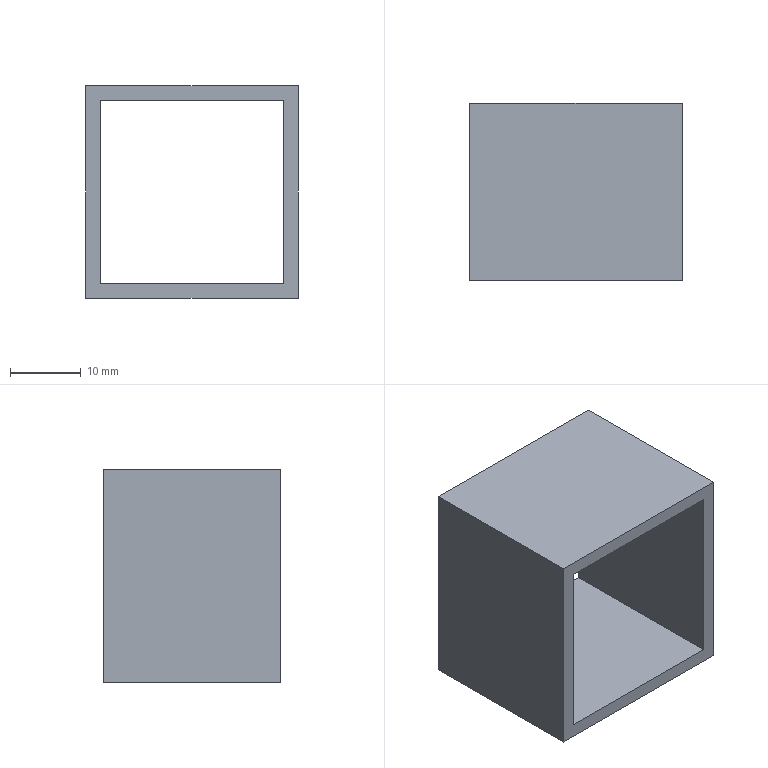Part | NX | features solid 2 | 1 solid | 10 faces | box 30 x 25 x 30 mm | volume 5600 mm3 | plane 10
STEP:
#1=CARTESIAN_POINT('',(350.,325.,-45.));
#2=VERTEX_POINT('',#1);
#3=CARTESIAN_POINT('',(380.,325.,-45.));
#4=VERTEX_POINT('',#3);
#5=CARTESIAN_POINT('',(350.,325.,-45.));
#6=DIRECTION('',(-1.,0.,0.));
#7=VECTOR('',#6,1000.);
#8=LINE('',#5,#7);
#9=EDGE_CURVE('',#2,#4,#8,.F.);
#10=ORIENTED_EDGE('',*,*,#9,.F.);
#11=CARTESIAN_POINT('',(350.,300.,-45.));
#12=VERTEX_POINT('',#11);
#13=CARTESIAN_POINT('',(350.,325.,-45.));
#14=DIRECTION('',(0.,-1.,0.));
#15=VECTOR('',#14,1000.);
#16=LINE('',#13,#15);
#17=EDGE_CURVE('',#2,#12,#16,.T.);
#18=ORIENTED_EDGE('',*,*,#17,.T.);
#19=CARTESIAN_POINT('',(380.,300.,-45.));
#20=VERTEX_POINT('',#19);
#21=CARTESIAN_POINT('',(350.,300.,-45.));
#22=DIRECTION('',(-1.,0.,0.));
#23=VECTOR('',#22,1000.);
#24=LINE('',#21,#23);
#25=EDGE_CURVE('',#12,#20,#24,.F.);
#26=ORIENTED_EDGE('',*,*,#25,.T.);
#27=CARTESIAN_POINT('',(380.,325.,-45.));
#28=DIRECTION('',(0.,-1.,0.));
#29=VECTOR('',#28,1000.);
#30=LINE('',#27,#29);
#31=EDGE_CURVE('',#4,#20,#30,.T.);
#32=ORIENTED_EDGE('',*,*,#31,.F.);
#33=EDGE_LOOP('',(#10,#18,#26,#32));
#34=FACE_BOUND('',#33,.T.);
#35=CARTESIAN_POINT('',(350.,325.,-45.));
#36=DIRECTION('',(0.,0.,-1.));
#37=DIRECTION('',(1.,0.,0.));
#38=AXIS2_PLACEMENT_3D('',#35,#36,#37);
#39=PLANE('',#38);
#40=ADVANCED_FACE('',(#34),#39,.F.);
#41=CARTESIAN_POINT('',(380.,325.,-75.));
#42=VERTEX_POINT('',#41);
#43=CARTESIAN_POINT('',(380.,325.,-45.));
#44=DIRECTION('',(0.,0.,1.));
#45=VECTOR('',#44,1000.);
#46=LINE('',#43,#45);
#47=EDGE_CURVE('',#4,#42,#46,.F.);
#48=ORIENTED_EDGE('',*,*,#47,.F.);
#49=ORIENTED_EDGE('',*,*,#31,.T.);
#50=CARTESIAN_POINT('',(380.,300.,-75.));
#51=VERTEX_POINT('',#50);
#52=CARTESIAN_POINT('',(380.,300.,-45.));
#53=DIRECTION('',(0.,0.,1.));
#54=VECTOR('',#53,1000.);
#55=LINE('',#52,#54);
#56=EDGE_CURVE('',#20,#51,#55,.F.);
#57=ORIENTED_EDGE('',*,*,#56,.T.);
#58=CARTESIAN_POINT('',(380.,325.,-75.));
#59=DIRECTION('',(0.,-1.,0.));
#60=VECTOR('',#59,1000.);
#61=LINE('',#58,#60);
#62=EDGE_CURVE('',#42,#51,#61,.T.);
#63=ORIENTED_EDGE('',*,*,#62,.F.);
#64=EDGE_LOOP('',(#48,#49,#57,#63));
#65=FACE_BOUND('',#64,.T.);
#66=CARTESIAN_POINT('',(380.,325.,-45.));
#67=DIRECTION('',(-1.,0.,0.));
#68=DIRECTION('',(0.,0.,-1.));
#69=AXIS2_PLACEMENT_3D('',#66,#67,#68);
#70=PLANE('',#69);
#71=ADVANCED_FACE('',(#65),#70,.F.);
#72=CARTESIAN_POINT('',(350.,325.,-75.));
#73=VERTEX_POINT('',#72);
#74=CARTESIAN_POINT('',(350.,325.,-75.));
#75=DIRECTION('',(-1.,0.,0.));
#76=VECTOR('',#75,1000.);
#77=LINE('',#74,#76);
#78=EDGE_CURVE('',#42,#73,#77,.T.);
#79=ORIENTED_EDGE('',*,*,#78,.F.);
#80=ORIENTED_EDGE('',*,*,#62,.T.);
#81=CARTESIAN_POINT('',(350.,300.,-75.));
#82=VERTEX_POINT('',#81);
#83=CARTESIAN_POINT('',(25.,300.,-75.));
#84=DIRECTION('',(1.,0.,0.));
#85=VECTOR('',#84,1000.);
#86=LINE('',#83,#85);
#87=EDGE_CURVE('',#82,#51,#86,.T.);
#88=ORIENTED_EDGE('',*,*,#87,.F.);
#89=CARTESIAN_POINT('',(350.,325.,-75.));
#90=DIRECTION('',(0.,-1.,0.));
#91=VECTOR('',#90,1000.);
#92=LINE('',#89,#91);
#93=EDGE_CURVE('',#73,#82,#92,.T.);
#94=ORIENTED_EDGE('',*,*,#93,.F.);
#95=EDGE_LOOP('',(#79,#80,#88,#94));
#96=FACE_BOUND('',#95,.T.);
#97=CARTESIAN_POINT('',(350.,325.,-75.));
#98=DIRECTION('',(0.,0.,-1.));
#99=DIRECTION('',(1.,0.,0.));
#100=AXIS2_PLACEMENT_3D('',#97,#98,#99);
#101=PLANE('',#100);
#102=ADVANCED_FACE('',(#96),#101,.T.);
#103=CARTESIAN_POINT('',(350.,325.,-45.));
#104=DIRECTION('',(0.,0.,1.));
#105=VECTOR('',#104,1000.);
#106=LINE('',#103,#105);
#107=EDGE_CURVE('',#73,#2,#106,.T.);
#108=ORIENTED_EDGE('',*,*,#107,.F.);
#109=ORIENTED_EDGE('',*,*,#93,.T.);
#110=CARTESIAN_POINT('',(350.,300.,-45.));
#111=DIRECTION('',(0.,0.,-1.));
#112=VECTOR('',#111,1000.);
#113=LINE('',#110,#112);
#114=EDGE_CURVE('',#12,#82,#113,.T.);
#115=ORIENTED_EDGE('',*,*,#114,.F.);
#116=ORIENTED_EDGE('',*,*,#17,.F.);
#117=EDGE_LOOP('',(#108,#109,#115,#116));
#118=FACE_BOUND('',#117,.T.);
#119=CARTESIAN_POINT('',(350.,325.,-45.));
#120=DIRECTION('',(-1.,0.,0.));
#121=DIRECTION('',(0.,0.,-1.));
#122=AXIS2_PLACEMENT_3D('',#119,#120,#121);
#123=PLANE('',#122);
#124=ADVANCED_FACE('',(#118),#123,.T.);
#125=ORIENTED_EDGE('',*,*,#56,.F.);
#126=ORIENTED_EDGE('',*,*,#25,.F.);
#127=ORIENTED_EDGE('',*,*,#114,.T.);
#128=ORIENTED_EDGE('',*,*,#87,.T.);
#129=EDGE_LOOP('',(#125,#126,#127,#128));
#130=FACE_BOUND('',#129,.T.);
#131=CARTESIAN_POINT('',(352.,300.,-47.));
#132=VERTEX_POINT('',#131);
#133=CARTESIAN_POINT('',(378.,300.,-47.));
#134=VERTEX_POINT('',#133);
#135=CARTESIAN_POINT('',(350.,300.,-47.));
#136=DIRECTION('',(-1.,0.,0.));
#137=VECTOR('',#136,1000.);
#138=LINE('',#135,#137);
#139=EDGE_CURVE('',#132,#134,#138,.F.);
#140=ORIENTED_EDGE('',*,*,#139,.T.);
#141=CARTESIAN_POINT('',(378.,300.,-73.));
#142=VERTEX_POINT('',#141);
#143=CARTESIAN_POINT('',(378.,300.,-45.));
#144=DIRECTION('',(0.,0.,1.));
#145=VECTOR('',#144,1000.);
#146=LINE('',#143,#145);
#147=EDGE_CURVE('',#134,#142,#146,.F.);
#148=ORIENTED_EDGE('',*,*,#147,.T.);
#149=CARTESIAN_POINT('',(352.,300.,-73.));
#150=VERTEX_POINT('',#149);
#151=CARTESIAN_POINT('',(25.,300.,-73.));
#152=DIRECTION('',(1.,0.,0.));
#153=VECTOR('',#152,1000.);
#154=LINE('',#151,#153);
#155=EDGE_CURVE('',#150,#142,#154,.T.);
#156=ORIENTED_EDGE('',*,*,#155,.F.);
#157=CARTESIAN_POINT('',(352.,300.,-45.));
#158=DIRECTION('',(0.,0.,-1.));
#159=VECTOR('',#158,1000.);
#160=LINE('',#157,#159);
#161=EDGE_CURVE('',#132,#150,#160,.T.);
#162=ORIENTED_EDGE('',*,*,#161,.F.);
#163=EDGE_LOOP('',(#140,#148,#156,#162));
#164=FACE_BOUND('',#163,.T.);
#165=CARTESIAN_POINT('',(25.,300.,-45.));
#166=DIRECTION('',(0.,-1.,0.));
#167=DIRECTION('',(1.,0.,0.));
#168=AXIS2_PLACEMENT_3D('',#165,#166,#167);
#169=PLANE('',#168);
#170=ADVANCED_FACE('',(#130,#164),#169,.T.);
#171=CARTESIAN_POINT('',(352.,325.,-47.));
#172=VERTEX_POINT('',#171);
#173=CARTESIAN_POINT('',(352.,325.,-47.));
#174=DIRECTION('',(0.,1.,0.));
#175=VECTOR('',#174,1000.);
#176=LINE('',#173,#175);
#177=EDGE_CURVE('',#172,#132,#176,.F.);
#178=ORIENTED_EDGE('',*,*,#177,.F.);
#179=CARTESIAN_POINT('',(378.,325.,-47.));
#180=VERTEX_POINT('',#179);
#181=CARTESIAN_POINT('',(350.,325.,-47.));
#182=DIRECTION('',(-1.,0.,0.));
#183=VECTOR('',#182,1000.);
#184=LINE('',#181,#183);
#185=EDGE_CURVE('',#172,#180,#184,.F.);
#186=ORIENTED_EDGE('',*,*,#185,.T.);
#187=CARTESIAN_POINT('',(378.,325.,-47.));
#188=DIRECTION('',(0.,-1.,0.));
#189=VECTOR('',#188,1000.);
#190=LINE('',#187,#189);
#191=EDGE_CURVE('',#180,#134,#190,.T.);
#192=ORIENTED_EDGE('',*,*,#191,.T.);
#193=ORIENTED_EDGE('',*,*,#139,.F.);
#194=EDGE_LOOP('',(#178,#186,#192,#193));
#195=FACE_BOUND('',#194,.T.);
#196=CARTESIAN_POINT('',(350.,325.,-47.));
#197=DIRECTION('',(0.,0.,-1.));
#198=DIRECTION('',(1.,0.,0.));
#199=AXIS2_PLACEMENT_3D('',#196,#197,#198);
#200=PLANE('',#199);
#201=ADVANCED_FACE('',(#195),#200,.T.);
#202=ORIENTED_EDGE('',*,*,#191,.F.);
#203=CARTESIAN_POINT('',(378.,325.,-73.));
#204=VERTEX_POINT('',#203);
#205=CARTESIAN_POINT('',(378.,325.,-45.));
#206=DIRECTION('',(0.,0.,1.));
#207=VECTOR('',#206,1000.);
#208=LINE('',#205,#207);
#209=EDGE_CURVE('',#180,#204,#208,.F.);
#210=ORIENTED_EDGE('',*,*,#209,.T.);
#211=CARTESIAN_POINT('',(378.,325.,-73.));
#212=DIRECTION('',(0.,1.,0.));
#213=VECTOR('',#212,1000.);
#214=LINE('',#211,#213);
#215=EDGE_CURVE('',#204,#142,#214,.F.);
#216=ORIENTED_EDGE('',*,*,#215,.T.);
#217=ORIENTED_EDGE('',*,*,#147,.F.);
#218=EDGE_LOOP('',(#202,#210,#216,#217));
#219=FACE_BOUND('',#218,.T.);
#220=CARTESIAN_POINT('',(378.,325.,-45.));
#221=DIRECTION('',(-1.,0.,0.));
#222=DIRECTION('',(0.,0.,-1.));
#223=AXIS2_PLACEMENT_3D('',#220,#221,#222);
#224=PLANE('',#223);
#225=ADVANCED_FACE('',(#219),#224,.T.);
#226=ORIENTED_EDGE('',*,*,#215,.F.);
#227=CARTESIAN_POINT('',(352.,325.,-73.));
#228=VERTEX_POINT('',#227);
#229=CARTESIAN_POINT('',(350.,325.,-73.));
#230=DIRECTION('',(-1.,0.,0.));
#231=VECTOR('',#230,1000.);
#232=LINE('',#229,#231);
#233=EDGE_CURVE('',#204,#228,#232,.T.);
#234=ORIENTED_EDGE('',*,*,#233,.T.);
#235=CARTESIAN_POINT('',(352.,325.,-73.));
#236=DIRECTION('',(0.,-1.,0.));
#237=VECTOR('',#236,1000.);
#238=LINE('',#235,#237);
#239=EDGE_CURVE('',#228,#150,#238,.T.);
#240=ORIENTED_EDGE('',*,*,#239,.T.);
#241=ORIENTED_EDGE('',*,*,#155,.T.);
#242=EDGE_LOOP('',(#226,#234,#240,#241));
#243=FACE_BOUND('',#242,.T.);
#244=CARTESIAN_POINT('',(350.,325.,-73.));
#245=DIRECTION('',(0.,0.,-1.));
#246=DIRECTION('',(1.,0.,0.));
#247=AXIS2_PLACEMENT_3D('',#244,#245,#246);
#248=PLANE('',#247);
#249=ADVANCED_FACE('',(#243),#248,.F.);
#250=ORIENTED_EDGE('',*,*,#239,.F.);
#251=CARTESIAN_POINT('',(352.,325.,-45.));
#252=DIRECTION('',(0.,0.,1.));
#253=VECTOR('',#252,1000.);
#254=LINE('',#251,#253);
#255=EDGE_CURVE('',#228,#172,#254,.T.);
#256=ORIENTED_EDGE('',*,*,#255,.T.);
#257=ORIENTED_EDGE('',*,*,#177,.T.);
#258=ORIENTED_EDGE('',*,*,#161,.T.);
#259=EDGE_LOOP('',(#250,#256,#257,#258));
#260=FACE_BOUND('',#259,.T.);
#261=CARTESIAN_POINT('',(352.,325.,-45.));
#262=DIRECTION('',(-1.,0.,0.));
#263=DIRECTION('',(0.,0.,-1.));
#264=AXIS2_PLACEMENT_3D('',#261,#262,#263);
#265=PLANE('',#264);
#266=ADVANCED_FACE('',(#260),#265,.F.);
#267=ORIENTED_EDGE('',*,*,#107,.T.);
#268=ORIENTED_EDGE('',*,*,#9,.T.);
#269=ORIENTED_EDGE('',*,*,#47,.T.);
#270=ORIENTED_EDGE('',*,*,#78,.T.);
#271=EDGE_LOOP('',(#267,#268,#269,#270));
#272=FACE_BOUND('',#271,.T.);
#273=ORIENTED_EDGE('',*,*,#233,.F.);
#274=ORIENTED_EDGE('',*,*,#209,.F.);
#275=ORIENTED_EDGE('',*,*,#185,.F.);
#276=ORIENTED_EDGE('',*,*,#255,.F.);
#277=EDGE_LOOP('',(#273,#274,#275,#276));
#278=FACE_BOUND('',#277,.T.);
#279=CARTESIAN_POINT('',(25.,325.,-75.));
#280=DIRECTION('',(0.,-1.,0.));
#281=DIRECTION('',(1.,0.,0.));
#282=AXIS2_PLACEMENT_3D('',#279,#280,#281);
#283=PLANE('',#282);
#284=ADVANCED_FACE('',(#272,#278),#283,.F.);
#285=CLOSED_SHELL('',(#40,#71,#102,#124,#170,#201,#225,#249,#266,#284));
#286=MANIFOLD_SOLID_BREP('',#285);
#287=(LENGTH_UNIT()NAMED_UNIT(*)SI_UNIT(.MILLI.,.METRE.));
#288=UNCERTAINTY_MEASURE_WITH_UNIT(LENGTH_MEASURE(0.00001),#287,'','');
#289=(NAMED_UNIT(*)PLANE_ANGLE_UNIT()SI_UNIT($,.RADIAN.));
#290=(NAMED_UNIT(*)SI_UNIT($,.STERADIAN.)SOLID_ANGLE_UNIT());
#291=(GEOMETRIC_REPRESENTATION_CONTEXT(3)GLOBAL_UNCERTAINTY_ASSIGNED_CONTEXT((#288))GLOBAL_UNIT_ASSIGNED_CONTEXT((#287,#289,#290))REPRESENTATION_CONTEXT('',''));
#292=ADVANCED_BREP_SHAPE_REPRESENTATION('',(#286),#291);